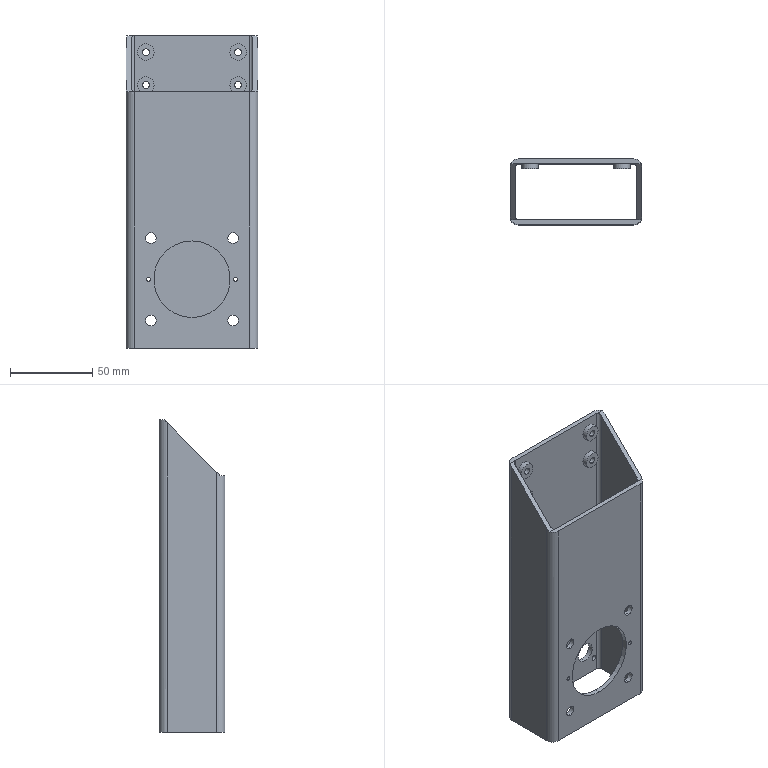Part | SolidWorks | features HoleWzd 5, ICE 4, Extrusion 1 | 1 solid | 75 faces | box 80 x 40 x 190 mm | volume 108540 mm3 | cylinder 58 | plane 17 | commonest cylinder face diameters 10 x12 3.3 x8 4.2 x8 6.5 x8 12 x8 2.5 x4